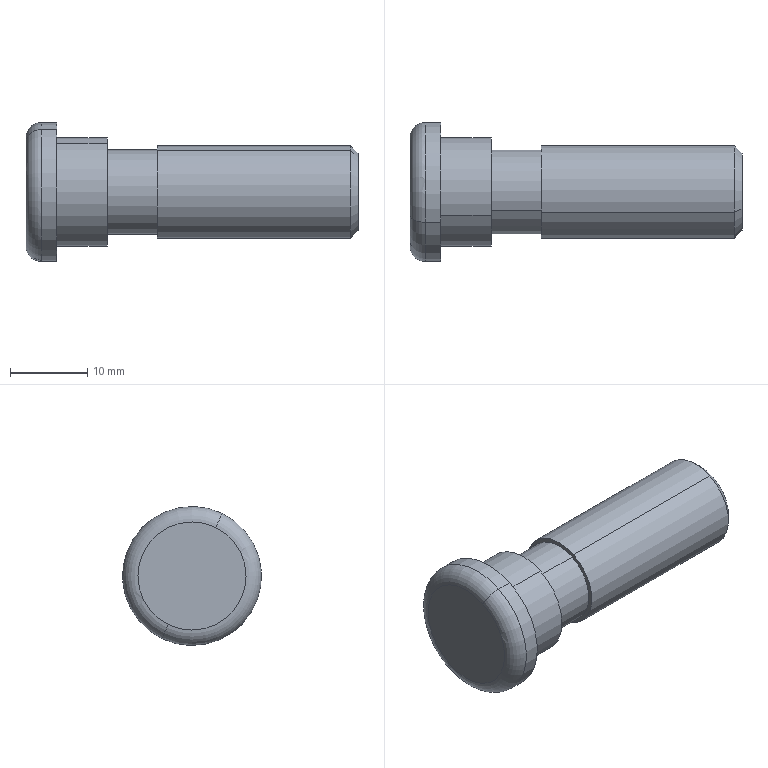Part | NX | features BREP 1 | 1 solid | 17 faces | box 43 x 18 x 18 mm | volume 5504 mm3 | cylinder 8 | plane 5 | torus 2 | cone 2 | commonest cylinder face diameters 10.92 x2 12 x2 14 x2 18 x2
STEP:
#1=CARTESIAN_POINT('',(766.132,18.282,53.036));
#2=VERTEX_POINT('',#1);
#3=CARTESIAN_POINT('',(766.132,23.517,42.238));
#4=VERTEX_POINT('',#3);
#5=CARTESIAN_POINT('',(766.132,20.899,47.637));
#6=DIRECTION('',(1.,0.,0.));
#7=DIRECTION('',(0.,-0.4362,0.8998));
#8=AXIS2_PLACEMENT_3D('',#5,#6,#7);
#9=CIRCLE('',#8,6.);
#10=EDGE_CURVE('',#2,#4,#9,.T.);
#11=ORIENTED_EDGE('',*,*,#10,.T.);
#12=CARTESIAN_POINT('',(791.132,23.517,42.238));
#13=VERTEX_POINT('',#12);
#14=CARTESIAN_POINT('',(792.132,23.517,42.238));
#15=DIRECTION('',(1.,0.,0.));
#16=VECTOR('',#15,1000.);
#17=LINE('',#14,#16);
#18=EDGE_CURVE('',#13,#4,#17,.F.);
#19=ORIENTED_EDGE('',*,*,#18,.F.);
#20=CARTESIAN_POINT('',(791.132,18.282,53.036));
#21=VERTEX_POINT('',#20);
#22=CARTESIAN_POINT('',(791.132,20.899,47.637));
#23=DIRECTION('',(1.,0.,0.));
#24=DIRECTION('',(0.,-0.4362,0.8998));
#25=AXIS2_PLACEMENT_3D('',#22,#23,#24);
#26=CIRCLE('',#25,6.);
#27=EDGE_CURVE('',#21,#13,#26,.T.);
#28=ORIENTED_EDGE('',*,*,#27,.F.);
#29=CARTESIAN_POINT('',(792.132,18.282,53.036));
#30=DIRECTION('',(1.,0.,0.));
#31=VECTOR('',#30,1000.);
#32=LINE('',#29,#31);
#33=EDGE_CURVE('',#21,#2,#32,.F.);
#34=ORIENTED_EDGE('',*,*,#33,.T.);
#35=EDGE_LOOP('',(#11,#19,#28,#34));
#36=FACE_BOUND('',#35,.T.);
#37=CARTESIAN_POINT('',(792.132,20.899,47.637));
#38=DIRECTION('',(1.,0.,0.));
#39=DIRECTION('',(0.,0.4362,-0.8998));
#40=AXIS2_PLACEMENT_3D('',#37,#38,#39);
#41=CYLINDRICAL_SURFACE('',#40,6.);
#42=ADVANCED_FACE('',(#36),#41,.T.);
#43=CARTESIAN_POINT('',(759.632,18.517,52.55));
#44=VERTEX_POINT('',#43);
#45=CARTESIAN_POINT('',(759.632,23.281,42.724));
#46=VERTEX_POINT('',#45);
#47=CARTESIAN_POINT('',(759.632,20.899,47.637));
#48=DIRECTION('',(1.,0.,0.));
#49=DIRECTION('',(0.,-0.4362,0.8998));
#50=AXIS2_PLACEMENT_3D('',#47,#48,#49);
#51=CIRCLE('',#50,5.46);
#52=EDGE_CURVE('',#44,#46,#51,.T.);
#53=ORIENTED_EDGE('',*,*,#52,.T.);
#54=CARTESIAN_POINT('',(766.132,23.281,42.724));
#55=VERTEX_POINT('',#54);
#56=CARTESIAN_POINT('',(792.132,23.281,42.724));
#57=DIRECTION('',(1.,0.,0.));
#58=VECTOR('',#57,1000.);
#59=LINE('',#56,#58);
#60=EDGE_CURVE('',#55,#46,#59,.F.);
#61=ORIENTED_EDGE('',*,*,#60,.F.);
#62=CARTESIAN_POINT('',(766.132,18.517,52.55));
#63=VERTEX_POINT('',#62);
#64=CARTESIAN_POINT('',(766.132,20.899,47.637));
#65=DIRECTION('',(1.,0.,0.));
#66=DIRECTION('',(0.,-0.4362,0.8998));
#67=AXIS2_PLACEMENT_3D('',#64,#65,#66);
#68=CIRCLE('',#67,5.46);
#69=EDGE_CURVE('',#63,#55,#68,.T.);
#70=ORIENTED_EDGE('',*,*,#69,.F.);
#71=CARTESIAN_POINT('',(792.132,18.517,52.55));
#72=DIRECTION('',(1.,0.,0.));
#73=VECTOR('',#72,1000.);
#74=LINE('',#71,#73);
#75=EDGE_CURVE('',#63,#44,#74,.F.);
#76=ORIENTED_EDGE('',*,*,#75,.T.);
#77=EDGE_LOOP('',(#53,#61,#70,#76));
#78=FACE_BOUND('',#77,.T.);
#79=CARTESIAN_POINT('',(792.132,20.899,47.637));
#80=DIRECTION('',(1.,0.,0.));
#81=DIRECTION('',(0.,0.4362,-0.8998));
#82=AXIS2_PLACEMENT_3D('',#79,#80,#81);
#83=CYLINDRICAL_SURFACE('',#82,5.46);
#84=ADVANCED_FACE('',(#78),#83,.T.);
#85=CARTESIAN_POINT('',(753.132,17.846,53.936));
#86=VERTEX_POINT('',#85);
#87=CARTESIAN_POINT('',(753.132,23.953,41.338));
#88=VERTEX_POINT('',#87);
#89=CARTESIAN_POINT('',(753.132,20.899,47.637));
#90=DIRECTION('',(1.,0.,0.));
#91=DIRECTION('',(0.,-0.4362,0.8998));
#92=AXIS2_PLACEMENT_3D('',#89,#90,#91);
#93=CIRCLE('',#92,7.);
#94=EDGE_CURVE('',#86,#88,#93,.T.);
#95=ORIENTED_EDGE('',*,*,#94,.T.);
#96=CARTESIAN_POINT('',(759.632,23.953,41.338));
#97=VERTEX_POINT('',#96);
#98=CARTESIAN_POINT('',(792.132,23.953,41.338));
#99=DIRECTION('',(1.,0.,0.));
#100=VECTOR('',#99,1000.);
#101=LINE('',#98,#100);
#102=EDGE_CURVE('',#97,#88,#101,.F.);
#103=ORIENTED_EDGE('',*,*,#102,.F.);
#104=CARTESIAN_POINT('',(759.632,17.846,53.936));
#105=VERTEX_POINT('',#104);
#106=CARTESIAN_POINT('',(759.632,20.899,47.637));
#107=DIRECTION('',(1.,0.,0.));
#108=DIRECTION('',(0.,-0.4362,0.8998));
#109=AXIS2_PLACEMENT_3D('',#106,#107,#108);
#110=CIRCLE('',#109,7.);
#111=EDGE_CURVE('',#105,#97,#110,.T.);
#112=ORIENTED_EDGE('',*,*,#111,.F.);
#113=CARTESIAN_POINT('',(792.132,17.846,53.936));
#114=DIRECTION('',(1.,0.,0.));
#115=VECTOR('',#114,1000.);
#116=LINE('',#113,#115);
#117=EDGE_CURVE('',#105,#86,#116,.F.);
#118=ORIENTED_EDGE('',*,*,#117,.T.);
#119=EDGE_LOOP('',(#95,#103,#112,#118));
#120=FACE_BOUND('',#119,.T.);
#121=CARTESIAN_POINT('',(792.132,20.899,47.637));
#122=DIRECTION('',(1.,0.,0.));
#123=DIRECTION('',(0.,0.4362,-0.8998));
#124=AXIS2_PLACEMENT_3D('',#121,#122,#123);
#125=CYLINDRICAL_SURFACE('',#124,7.);
#126=ADVANCED_FACE('',(#120),#125,.T.);
#127=CARTESIAN_POINT('',(751.132,16.973,55.736));
#128=VERTEX_POINT('',#127);
#129=CARTESIAN_POINT('',(751.132,24.825,39.539));
#130=VERTEX_POINT('',#129);
#131=CARTESIAN_POINT('',(751.132,20.899,47.637));
#132=DIRECTION('',(1.,0.,0.));
#133=DIRECTION('',(0.,-0.4362,0.8998));
#134=AXIS2_PLACEMENT_3D('',#131,#132,#133);
#135=CIRCLE('',#134,9.);
#136=EDGE_CURVE('',#128,#130,#135,.T.);
#137=ORIENTED_EDGE('',*,*,#136,.T.);
#138=CARTESIAN_POINT('',(753.132,24.825,39.539));
#139=VERTEX_POINT('',#138);
#140=CARTESIAN_POINT('',(792.132,24.825,39.539));
#141=DIRECTION('',(1.,0.,0.));
#142=VECTOR('',#141,1000.);
#143=LINE('',#140,#142);
#144=EDGE_CURVE('',#139,#130,#143,.F.);
#145=ORIENTED_EDGE('',*,*,#144,.F.);
#146=CARTESIAN_POINT('',(753.132,16.973,55.736));
#147=VERTEX_POINT('',#146);
#148=CARTESIAN_POINT('',(753.132,20.899,47.637));
#149=DIRECTION('',(1.,0.,0.));
#150=DIRECTION('',(0.,-0.4362,0.8998));
#151=AXIS2_PLACEMENT_3D('',#148,#149,#150);
#152=CIRCLE('',#151,9.);
#153=EDGE_CURVE('',#147,#139,#152,.T.);
#154=ORIENTED_EDGE('',*,*,#153,.F.);
#155=CARTESIAN_POINT('',(792.132,16.973,55.736));
#156=DIRECTION('',(1.,0.,0.));
#157=VECTOR('',#156,1000.);
#158=LINE('',#155,#157);
#159=EDGE_CURVE('',#147,#128,#158,.F.);
#160=ORIENTED_EDGE('',*,*,#159,.T.);
#161=EDGE_LOOP('',(#137,#145,#154,#160));
#162=FACE_BOUND('',#161,.T.);
#163=CARTESIAN_POINT('',(792.132,20.899,47.637));
#164=DIRECTION('',(1.,0.,0.));
#165=DIRECTION('',(0.,0.4362,-0.8998));
#166=AXIS2_PLACEMENT_3D('',#163,#164,#165);
#167=CYLINDRICAL_SURFACE('',#166,9.);
#168=ADVANCED_FACE('',(#162),#167,.T.);
#169=CARTESIAN_POINT('',(749.132,17.846,53.936));
#170=VERTEX_POINT('',#169);
#171=CARTESIAN_POINT('',(749.132,23.953,41.338));
#172=VERTEX_POINT('',#171);
#173=CARTESIAN_POINT('',(749.132,20.899,47.637));
#174=DIRECTION('',(1.,0.,0.));
#175=DIRECTION('',(0.,-0.4362,0.8998));
#176=AXIS2_PLACEMENT_3D('',#173,#174,#175);
#177=CIRCLE('',#176,7.);
#178=EDGE_CURVE('',#170,#172,#177,.T.);
#179=ORIENTED_EDGE('',*,*,#178,.T.);
#180=CARTESIAN_POINT('',(751.132,23.953,41.338));
#181=DIRECTION('',(0.,-0.8998,-0.4362));
#182=DIRECTION('',(0.,0.4362,-0.8998));
#183=AXIS2_PLACEMENT_3D('',#180,#181,#182);
#184=CIRCLE('',#183,2.);
#185=EDGE_CURVE('',#130,#172,#184,.F.);
#186=ORIENTED_EDGE('',*,*,#185,.F.);
#187=ORIENTED_EDGE('',*,*,#136,.F.);
#188=CARTESIAN_POINT('',(751.132,17.846,53.936));
#189=DIRECTION('',(0.,0.8998,0.4362));
#190=DIRECTION('',(0.,-0.4362,0.8998));
#191=AXIS2_PLACEMENT_3D('',#188,#189,#190);
#192=CIRCLE('',#191,2.);
#193=EDGE_CURVE('',#128,#170,#192,.F.);
#194=ORIENTED_EDGE('',*,*,#193,.T.);
#195=EDGE_LOOP('',(#179,#186,#187,#194));
#196=FACE_BOUND('',#195,.T.);
#197=CARTESIAN_POINT('',(751.132,20.899,47.637));
#198=DIRECTION('',(1.,0.,0.));
#199=DIRECTION('',(0.,0.4362,-0.8998));
#200=AXIS2_PLACEMENT_3D('',#197,#198,#199);
#201=TOROIDAL_SURFACE('',#200,7.,2.);
#202=ADVANCED_FACE('',(#196),#201,.T.);
#203=CARTESIAN_POINT('',(792.132,18.718,52.136));
#204=VERTEX_POINT('',#203);
#205=CARTESIAN_POINT('',(792.132,23.08,43.138));
#206=VERTEX_POINT('',#205);
#207=CARTESIAN_POINT('',(792.132,20.899,47.637));
#208=DIRECTION('',(1.,0.,0.));
#209=DIRECTION('',(0.,-0.4362,0.8998));
#210=AXIS2_PLACEMENT_3D('',#207,#208,#209);
#211=CIRCLE('',#210,5.);
#212=EDGE_CURVE('',#204,#206,#211,.T.);
#213=ORIENTED_EDGE('',*,*,#212,.F.);
#214=CARTESIAN_POINT('',(791.132,18.282,53.036));
#215=DIRECTION('',(-0.7071,-0.3085,0.6363));
#216=VECTOR('',#215,1000.);
#217=LINE('',#214,#216);
#218=EDGE_CURVE('',#204,#21,#217,.T.);
#219=ORIENTED_EDGE('',*,*,#218,.T.);
#220=ORIENTED_EDGE('',*,*,#27,.T.);
#221=CARTESIAN_POINT('',(791.132,23.517,42.238));
#222=DIRECTION('',(-0.7071,0.3085,-0.6363));
#223=VECTOR('',#222,1000.);
#224=LINE('',#221,#223);
#225=EDGE_CURVE('',#206,#13,#224,.T.);
#226=ORIENTED_EDGE('',*,*,#225,.F.);
#227=EDGE_LOOP('',(#213,#219,#220,#226));
#228=FACE_BOUND('',#227,.T.);
#229=CARTESIAN_POINT('',(791.132,20.899,47.637));
#230=DIRECTION('',(-1.,0.,0.));
#231=DIRECTION('',(0.,-0.4362,0.8998));
#232=AXIS2_PLACEMENT_3D('',#229,#230,#231);
#233=CONICAL_SURFACE('',#232,6.,0.7854);
#234=ADVANCED_FACE('',(#228),#233,.T.);
#235=ORIENTED_EDGE('',*,*,#218,.F.);
#236=CARTESIAN_POINT('',(792.132,20.899,47.637));
#237=DIRECTION('',(1.,0.,0.));
#238=DIRECTION('',(0.,-0.4362,0.8998));
#239=AXIS2_PLACEMENT_3D('',#236,#237,#238);
#240=CIRCLE('',#239,5.);
#241=EDGE_CURVE('',#206,#204,#240,.T.);
#242=ORIENTED_EDGE('',*,*,#241,.F.);
#243=ORIENTED_EDGE('',*,*,#225,.T.);
#244=CARTESIAN_POINT('',(791.132,20.899,47.637));
#245=DIRECTION('',(1.,0.,0.));
#246=DIRECTION('',(0.,-0.4362,0.8998));
#247=AXIS2_PLACEMENT_3D('',#244,#245,#246);
#248=CIRCLE('',#247,6.);
#249=EDGE_CURVE('',#13,#21,#248,.T.);
#250=ORIENTED_EDGE('',*,*,#249,.T.);
#251=EDGE_LOOP('',(#235,#242,#243,#250));
#252=FACE_BOUND('',#251,.T.);
#253=CARTESIAN_POINT('',(791.132,20.899,47.637));
#254=DIRECTION('',(-1.,0.,0.));
#255=DIRECTION('',(0.,-0.4362,0.8998));
#256=AXIS2_PLACEMENT_3D('',#253,#254,#255);
#257=CONICAL_SURFACE('',#256,6.,0.7854);
#258=ADVANCED_FACE('',(#252),#257,.T.);
#259=ORIENTED_EDGE('',*,*,#241,.T.);
#260=ORIENTED_EDGE('',*,*,#212,.T.);
#261=EDGE_LOOP('',(#259,#260));
#262=FACE_BOUND('',#261,.T.);
#263=CARTESIAN_POINT('',(792.132,25.398,49.818));
#264=DIRECTION('',(-1.,0.,0.));
#265=DIRECTION('',(0.,-0.4362,0.8998));
#266=AXIS2_PLACEMENT_3D('',#263,#264,#265);
#267=PLANE('',#266);
#268=ADVANCED_FACE('',(#262),#267,.F.);
#269=ORIENTED_EDGE('',*,*,#178,.F.);
#270=CARTESIAN_POINT('',(749.132,20.899,47.637));
#271=DIRECTION('',(1.,0.,0.));
#272=DIRECTION('',(0.,-0.4362,0.8998));
#273=AXIS2_PLACEMENT_3D('',#270,#271,#272);
#274=CIRCLE('',#273,7.);
#275=EDGE_CURVE('',#172,#170,#274,.T.);
#276=ORIENTED_EDGE('',*,*,#275,.F.);
#277=EDGE_LOOP('',(#269,#276));
#278=FACE_BOUND('',#277,.T.);
#279=CARTESIAN_POINT('',(749.132,20.899,47.637));
#280=DIRECTION('',(1.,0.,0.));
#281=DIRECTION('',(0.,0.4362,-0.8998));
#282=AXIS2_PLACEMENT_3D('',#279,#280,#281);
#283=PLANE('',#282);
#284=ADVANCED_FACE('',(#278),#283,.F.);
#285=ORIENTED_EDGE('',*,*,#185,.T.);
#286=ORIENTED_EDGE('',*,*,#275,.T.);
#287=ORIENTED_EDGE('',*,*,#193,.F.);
#288=CARTESIAN_POINT('',(751.132,20.899,47.637));
#289=DIRECTION('',(1.,0.,0.));
#290=DIRECTION('',(0.,-0.4362,0.8998));
#291=AXIS2_PLACEMENT_3D('',#288,#289,#290);
#292=CIRCLE('',#291,9.);
#293=EDGE_CURVE('',#130,#128,#292,.T.);
#294=ORIENTED_EDGE('',*,*,#293,.F.);
#295=EDGE_LOOP('',(#285,#286,#287,#294));
#296=FACE_BOUND('',#295,.T.);
#297=CARTESIAN_POINT('',(751.132,20.899,47.637));
#298=DIRECTION('',(1.,0.,0.));
#299=DIRECTION('',(0.,0.4362,-0.8998));
#300=AXIS2_PLACEMENT_3D('',#297,#298,#299);
#301=TOROIDAL_SURFACE('',#300,7.,2.);
#302=ADVANCED_FACE('',(#296),#301,.T.);
#303=ORIENTED_EDGE('',*,*,#144,.T.);
#304=ORIENTED_EDGE('',*,*,#293,.T.);
#305=ORIENTED_EDGE('',*,*,#159,.F.);
#306=CARTESIAN_POINT('',(753.132,20.899,47.637));
#307=DIRECTION('',(1.,0.,0.));
#308=DIRECTION('',(0.,-0.4362,0.8998));
#309=AXIS2_PLACEMENT_3D('',#306,#307,#308);
#310=CIRCLE('',#309,9.);
#311=EDGE_CURVE('',#139,#147,#310,.T.);
#312=ORIENTED_EDGE('',*,*,#311,.F.);
#313=EDGE_LOOP('',(#303,#304,#305,#312));
#314=FACE_BOUND('',#313,.T.);
#315=CARTESIAN_POINT('',(792.132,20.899,47.637));
#316=DIRECTION('',(1.,0.,0.));
#317=DIRECTION('',(0.,0.4362,-0.8998));
#318=AXIS2_PLACEMENT_3D('',#315,#316,#317);
#319=CYLINDRICAL_SURFACE('',#318,9.);
#320=ADVANCED_FACE('',(#314),#319,.T.);
#321=ORIENTED_EDGE('',*,*,#94,.F.);
#322=CARTESIAN_POINT('',(753.132,20.899,47.637));
#323=DIRECTION('',(1.,0.,0.));
#324=DIRECTION('',(0.,-0.4362,0.8998));
#325=AXIS2_PLACEMENT_3D('',#322,#323,#324);
#326=CIRCLE('',#325,7.);
#327=EDGE_CURVE('',#88,#86,#326,.T.);
#328=ORIENTED_EDGE('',*,*,#327,.F.);
#329=EDGE_LOOP('',(#321,#328));
#330=FACE_BOUND('',#329,.T.);
#331=ORIENTED_EDGE('',*,*,#153,.T.);
#332=ORIENTED_EDGE('',*,*,#311,.T.);
#333=EDGE_LOOP('',(#331,#332));
#334=FACE_BOUND('',#333,.T.);
#335=CARTESIAN_POINT('',(753.132,28.998,51.563));
#336=DIRECTION('',(-1.,0.,0.));
#337=DIRECTION('',(0.,-0.4362,0.8998));
#338=AXIS2_PLACEMENT_3D('',#335,#336,#337);
#339=PLANE('',#338);
#340=ADVANCED_FACE('',(#330,#334),#339,.F.);
#341=ORIENTED_EDGE('',*,*,#102,.T.);
#342=ORIENTED_EDGE('',*,*,#327,.T.);
#343=ORIENTED_EDGE('',*,*,#117,.F.);
#344=CARTESIAN_POINT('',(759.632,20.899,47.637));
#345=DIRECTION('',(1.,0.,0.));
#346=DIRECTION('',(0.,-0.4362,0.8998));
#347=AXIS2_PLACEMENT_3D('',#344,#345,#346);
#348=CIRCLE('',#347,7.);
#349=EDGE_CURVE('',#97,#105,#348,.T.);
#350=ORIENTED_EDGE('',*,*,#349,.F.);
#351=EDGE_LOOP('',(#341,#342,#343,#350));
#352=FACE_BOUND('',#351,.T.);
#353=CARTESIAN_POINT('',(792.132,20.899,47.637));
#354=DIRECTION('',(1.,0.,0.));
#355=DIRECTION('',(0.,0.4362,-0.8998));
#356=AXIS2_PLACEMENT_3D('',#353,#354,#355);
#357=CYLINDRICAL_SURFACE('',#356,7.);
#358=ADVANCED_FACE('',(#352),#357,.T.);
#359=ORIENTED_EDGE('',*,*,#52,.F.);
#360=CARTESIAN_POINT('',(759.632,20.899,47.637));
#361=DIRECTION('',(1.,0.,0.));
#362=DIRECTION('',(0.,-0.4362,0.8998));
#363=AXIS2_PLACEMENT_3D('',#360,#361,#362);
#364=CIRCLE('',#363,5.46);
#365=EDGE_CURVE('',#46,#44,#364,.T.);
#366=ORIENTED_EDGE('',*,*,#365,.F.);
#367=EDGE_LOOP('',(#359,#366));
#368=FACE_BOUND('',#367,.T.);
#369=ORIENTED_EDGE('',*,*,#111,.T.);
#370=ORIENTED_EDGE('',*,*,#349,.T.);
#371=EDGE_LOOP('',(#369,#370));
#372=FACE_BOUND('',#371,.T.);
#373=CARTESIAN_POINT('',(759.632,27.198,50.691));
#374=DIRECTION('',(-1.,0.,0.));
#375=DIRECTION('',(0.,-0.4362,0.8998));
#376=AXIS2_PLACEMENT_3D('',#373,#374,#375);
#377=PLANE('',#376);
#378=ADVANCED_FACE('',(#368,#372),#377,.F.);
#379=ORIENTED_EDGE('',*,*,#60,.T.);
#380=ORIENTED_EDGE('',*,*,#365,.T.);
#381=ORIENTED_EDGE('',*,*,#75,.F.);
#382=CARTESIAN_POINT('',(766.132,20.899,47.637));
#383=DIRECTION('',(1.,0.,0.));
#384=DIRECTION('',(0.,-0.4362,0.8998));
#385=AXIS2_PLACEMENT_3D('',#382,#383,#384);
#386=CIRCLE('',#385,5.46);
#387=EDGE_CURVE('',#55,#63,#386,.T.);
#388=ORIENTED_EDGE('',*,*,#387,.F.);
#389=EDGE_LOOP('',(#379,#380,#381,#388));
#390=FACE_BOUND('',#389,.T.);
#391=CARTESIAN_POINT('',(792.132,20.899,47.637));
#392=DIRECTION('',(1.,0.,0.));
#393=DIRECTION('',(0.,0.4362,-0.8998));
#394=AXIS2_PLACEMENT_3D('',#391,#392,#393);
#395=CYLINDRICAL_SURFACE('',#394,5.46);
#396=ADVANCED_FACE('',(#390),#395,.T.);
#397=ORIENTED_EDGE('',*,*,#10,.F.);
#398=CARTESIAN_POINT('',(766.132,20.899,47.637));
#399=DIRECTION('',(1.,0.,0.));
#400=DIRECTION('',(0.,-0.4362,0.8998));
#401=AXIS2_PLACEMENT_3D('',#398,#399,#400);
#402=CIRCLE('',#401,6.);
#403=EDGE_CURVE('',#4,#2,#402,.T.);
#404=ORIENTED_EDGE('',*,*,#403,.F.);
#405=EDGE_LOOP('',(#397,#404));
#406=FACE_BOUND('',#405,.T.);
#407=ORIENTED_EDGE('',*,*,#69,.T.);
#408=ORIENTED_EDGE('',*,*,#387,.T.);
#409=EDGE_LOOP('',(#407,#408));
#410=FACE_BOUND('',#409,.T.);
#411=CARTESIAN_POINT('',(766.132,25.812,50.019));
#412=DIRECTION('',(1.,0.,0.));
#413=DIRECTION('',(0.,0.4362,-0.8998));
#414=AXIS2_PLACEMENT_3D('',#411,#412,#413);
#415=PLANE('',#414);
#416=ADVANCED_FACE('',(#406,#410),#415,.F.);
#417=ORIENTED_EDGE('',*,*,#18,.T.);
#418=ORIENTED_EDGE('',*,*,#403,.T.);
#419=ORIENTED_EDGE('',*,*,#33,.F.);
#420=ORIENTED_EDGE('',*,*,#249,.F.);
#421=EDGE_LOOP('',(#417,#418,#419,#420));
#422=FACE_BOUND('',#421,.T.);
#423=CARTESIAN_POINT('',(792.132,20.899,47.637));
#424=DIRECTION('',(1.,0.,0.));
#425=DIRECTION('',(0.,0.4362,-0.8998));
#426=AXIS2_PLACEMENT_3D('',#423,#424,#425);
#427=CYLINDRICAL_SURFACE('',#426,6.);
#428=ADVANCED_FACE('',(#422),#427,.T.);
#429=CLOSED_SHELL('',(#42,#84,#126,#168,#202,#234,#258,#268,#284,#302,#320,#340,#358,#378,#396,#416,#428));
#430=MANIFOLD_SOLID_BREP('',#429);
#431=(LENGTH_UNIT()NAMED_UNIT(*)SI_UNIT(.MILLI.,.METRE.));
#432=UNCERTAINTY_MEASURE_WITH_UNIT(LENGTH_MEASURE(0.00001),#431,'','');
#433=(NAMED_UNIT(*)PLANE_ANGLE_UNIT()SI_UNIT($,.RADIAN.));
#434=(NAMED_UNIT(*)SI_UNIT($,.STERADIAN.)SOLID_ANGLE_UNIT());
#435=(GEOMETRIC_REPRESENTATION_CONTEXT(3)GLOBAL_UNCERTAINTY_ASSIGNED_CONTEXT((#432))GLOBAL_UNIT_ASSIGNED_CONTEXT((#431,#433,#434))REPRESENTATION_CONTEXT('',''));
#436=ADVANCED_BREP_SHAPE_REPRESENTATION('',(#430),#435);